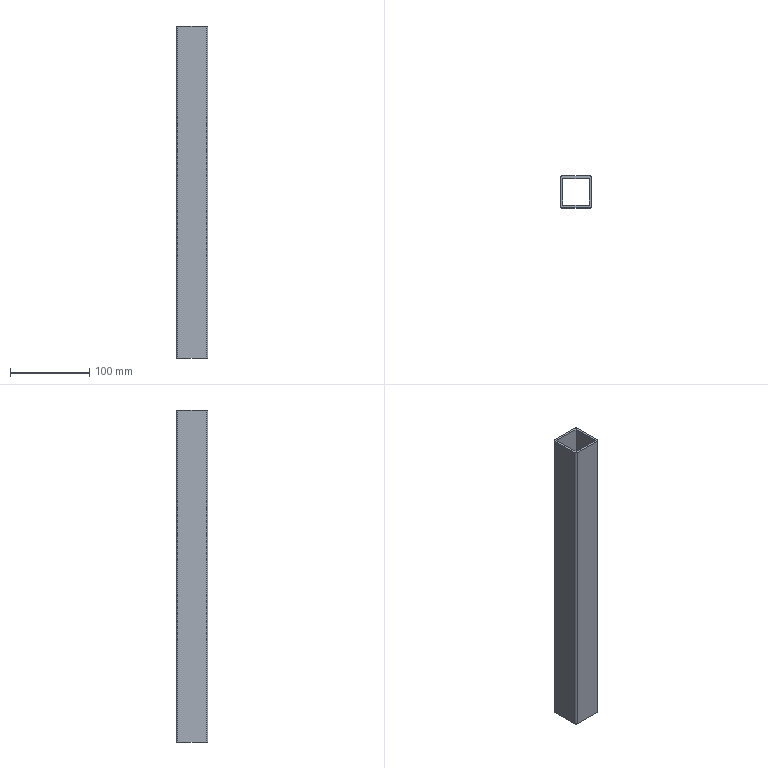Part | STEP file | X77-09108 | 1 solid | 14 faces | box 40 x 40 x 420 mm | volume 185038 mm3 | plane 10 | cylinder 4 | commonest cylinder face diameters 4 x4
STEP:
#1=CARTESIAN_POINT('',(0.,2.,420.));
#2=VERTEX_POINT('',#1);
#3=CARTESIAN_POINT('',(2.,0.,420.));
#4=VERTEX_POINT('',#3);
#5=CARTESIAN_POINT('',(2.,2.,420.));
#6=DIRECTION('',(0.,0.,1.));
#7=DIRECTION('',(1.,0.,0.));
#8=AXIS2_PLACEMENT_3D('',#5,#6,#7);
#9=CIRCLE('',#8,2.);
#10=EDGE_CURVE('',#2,#4,#9,.T.);
#11=ORIENTED_EDGE('',*,*,#10,.T.);
#12=CARTESIAN_POINT('',(38.,0.,420.));
#13=VERTEX_POINT('',#12);
#14=CARTESIAN_POINT('',(2.,0.,420.));
#15=DIRECTION('',(1.,0.,0.));
#16=VECTOR('',#15,1000.);
#17=LINE('',#14,#16);
#18=EDGE_CURVE('',#4,#13,#17,.T.);
#19=ORIENTED_EDGE('',*,*,#18,.T.);
#20=CARTESIAN_POINT('',(40.,2.,420.));
#21=VERTEX_POINT('',#20);
#22=CARTESIAN_POINT('',(38.,2.,420.));
#23=DIRECTION('',(0.,0.,1.));
#24=DIRECTION('',(1.,0.,0.));
#25=AXIS2_PLACEMENT_3D('',#22,#23,#24);
#26=CIRCLE('',#25,2.);
#27=EDGE_CURVE('',#13,#21,#26,.T.);
#28=ORIENTED_EDGE('',*,*,#27,.T.);
#29=CARTESIAN_POINT('',(40.,38.,420.));
#30=VERTEX_POINT('',#29);
#31=CARTESIAN_POINT('',(40.,2.,420.));
#32=DIRECTION('',(0.,1.,0.));
#33=VECTOR('',#32,1000.);
#34=LINE('',#31,#33);
#35=EDGE_CURVE('',#21,#30,#34,.T.);
#36=ORIENTED_EDGE('',*,*,#35,.T.);
#37=CARTESIAN_POINT('',(38.,40.,420.));
#38=VERTEX_POINT('',#37);
#39=CARTESIAN_POINT('',(38.,38.,420.));
#40=DIRECTION('',(0.,0.,1.));
#41=DIRECTION('',(1.,0.,0.));
#42=AXIS2_PLACEMENT_3D('',#39,#40,#41);
#43=CIRCLE('',#42,2.);
#44=EDGE_CURVE('',#30,#38,#43,.T.);
#45=ORIENTED_EDGE('',*,*,#44,.T.);
#46=CARTESIAN_POINT('',(2.,40.,420.));
#47=VERTEX_POINT('',#46);
#48=CARTESIAN_POINT('',(2.,40.,420.));
#49=DIRECTION('',(-1.,0.,0.));
#50=VECTOR('',#49,1000.);
#51=LINE('',#48,#50);
#52=EDGE_CURVE('',#38,#47,#51,.T.);
#53=ORIENTED_EDGE('',*,*,#52,.T.);
#54=CARTESIAN_POINT('',(0.,38.,420.));
#55=VERTEX_POINT('',#54);
#56=CARTESIAN_POINT('',(2.,38.,420.));
#57=DIRECTION('',(0.,0.,1.));
#58=DIRECTION('',(-1.,0.,0.));
#59=AXIS2_PLACEMENT_3D('',#56,#57,#58);
#60=CIRCLE('',#59,2.);
#61=EDGE_CURVE('',#47,#55,#60,.T.);
#62=ORIENTED_EDGE('',*,*,#61,.T.);
#63=CARTESIAN_POINT('',(0.,2.,420.));
#64=DIRECTION('',(0.,-1.,0.));
#65=VECTOR('',#64,1000.);
#66=LINE('',#63,#65);
#67=EDGE_CURVE('',#55,#2,#66,.T.);
#68=ORIENTED_EDGE('',*,*,#67,.T.);
#69=EDGE_LOOP('',(#11,#19,#28,#36,#45,#53,#62,#68));
#70=FACE_OUTER_BOUND('',#69,.T.);
#71=CARTESIAN_POINT('',(3.,3.,420.));
#72=VERTEX_POINT('',#71);
#73=CARTESIAN_POINT('',(37.,3.,420.));
#74=VERTEX_POINT('',#73);
#75=CARTESIAN_POINT('',(3.,3.,420.));
#76=DIRECTION('',(1.,0.,0.));
#77=VECTOR('',#76,1000.);
#78=LINE('',#75,#77);
#79=EDGE_CURVE('',#72,#74,#78,.T.);
#80=ORIENTED_EDGE('',*,*,#79,.F.);
#81=CARTESIAN_POINT('',(3.,37.,420.));
#82=VERTEX_POINT('',#81);
#83=CARTESIAN_POINT('',(3.,3.,420.));
#84=DIRECTION('',(0.,-1.,0.));
#85=VECTOR('',#84,1000.);
#86=LINE('',#83,#85);
#87=EDGE_CURVE('',#82,#72,#86,.T.);
#88=ORIENTED_EDGE('',*,*,#87,.F.);
#89=CARTESIAN_POINT('',(37.,37.,420.));
#90=VERTEX_POINT('',#89);
#91=CARTESIAN_POINT('',(3.,37.,420.));
#92=DIRECTION('',(-1.,0.,0.));
#93=VECTOR('',#92,1000.);
#94=LINE('',#91,#93);
#95=EDGE_CURVE('',#90,#82,#94,.T.);
#96=ORIENTED_EDGE('',*,*,#95,.F.);
#97=CARTESIAN_POINT('',(37.,3.,420.));
#98=DIRECTION('',(0.,1.,0.));
#99=VECTOR('',#98,1000.);
#100=LINE('',#97,#99);
#101=EDGE_CURVE('',#74,#90,#100,.T.);
#102=ORIENTED_EDGE('',*,*,#101,.F.);
#103=EDGE_LOOP('',(#80,#88,#96,#102));
#104=FACE_BOUND('',#103,.T.);
#105=CARTESIAN_POINT('',(2.,2.,420.));
#106=DIRECTION('',(0.,0.,1.));
#107=DIRECTION('',(1.,0.,0.));
#108=AXIS2_PLACEMENT_3D('',#105,#106,#107);
#109=PLANE('',#108);
#110=ADVANCED_FACE('',(#70,#104),#109,.T.);
#111=CARTESIAN_POINT('',(0.,2.,0.));
#112=VERTEX_POINT('',#111);
#113=CARTESIAN_POINT('',(2.,0.,0.));
#114=VERTEX_POINT('',#113);
#115=CARTESIAN_POINT('',(2.,2.,0.));
#116=DIRECTION('',(0.,0.,1.));
#117=DIRECTION('',(1.,0.,0.));
#118=AXIS2_PLACEMENT_3D('',#115,#116,#117);
#119=CIRCLE('',#118,2.);
#120=EDGE_CURVE('',#112,#114,#119,.T.);
#121=ORIENTED_EDGE('',*,*,#120,.F.);
#122=CARTESIAN_POINT('',(0.,38.,0.));
#123=VERTEX_POINT('',#122);
#124=CARTESIAN_POINT('',(0.,2.,0.));
#125=DIRECTION('',(0.,-1.,0.));
#126=VECTOR('',#125,1000.);
#127=LINE('',#124,#126);
#128=EDGE_CURVE('',#123,#112,#127,.T.);
#129=ORIENTED_EDGE('',*,*,#128,.F.);
#130=CARTESIAN_POINT('',(2.,40.,0.));
#131=VERTEX_POINT('',#130);
#132=CARTESIAN_POINT('',(2.,38.,0.));
#133=DIRECTION('',(0.,0.,1.));
#134=DIRECTION('',(-1.,0.,0.));
#135=AXIS2_PLACEMENT_3D('',#132,#133,#134);
#136=CIRCLE('',#135,2.);
#137=EDGE_CURVE('',#131,#123,#136,.T.);
#138=ORIENTED_EDGE('',*,*,#137,.F.);
#139=CARTESIAN_POINT('',(38.,40.,0.));
#140=VERTEX_POINT('',#139);
#141=CARTESIAN_POINT('',(2.,40.,0.));
#142=DIRECTION('',(-1.,0.,0.));
#143=VECTOR('',#142,1000.);
#144=LINE('',#141,#143);
#145=EDGE_CURVE('',#140,#131,#144,.T.);
#146=ORIENTED_EDGE('',*,*,#145,.F.);
#147=CARTESIAN_POINT('',(40.,38.,0.));
#148=VERTEX_POINT('',#147);
#149=CARTESIAN_POINT('',(38.,38.,0.));
#150=DIRECTION('',(0.,0.,1.));
#151=DIRECTION('',(1.,0.,0.));
#152=AXIS2_PLACEMENT_3D('',#149,#150,#151);
#153=CIRCLE('',#152,2.);
#154=EDGE_CURVE('',#148,#140,#153,.T.);
#155=ORIENTED_EDGE('',*,*,#154,.F.);
#156=CARTESIAN_POINT('',(40.,2.,0.));
#157=VERTEX_POINT('',#156);
#158=CARTESIAN_POINT('',(40.,2.,0.));
#159=DIRECTION('',(0.,1.,0.));
#160=VECTOR('',#159,1000.);
#161=LINE('',#158,#160);
#162=EDGE_CURVE('',#157,#148,#161,.T.);
#163=ORIENTED_EDGE('',*,*,#162,.F.);
#164=CARTESIAN_POINT('',(38.,0.,0.));
#165=VERTEX_POINT('',#164);
#166=CARTESIAN_POINT('',(38.,2.,0.));
#167=DIRECTION('',(0.,0.,1.));
#168=DIRECTION('',(1.,0.,0.));
#169=AXIS2_PLACEMENT_3D('',#166,#167,#168);
#170=CIRCLE('',#169,2.);
#171=EDGE_CURVE('',#165,#157,#170,.T.);
#172=ORIENTED_EDGE('',*,*,#171,.F.);
#173=CARTESIAN_POINT('',(2.,0.,0.));
#174=DIRECTION('',(1.,0.,0.));
#175=VECTOR('',#174,1000.);
#176=LINE('',#173,#175);
#177=EDGE_CURVE('',#114,#165,#176,.T.);
#178=ORIENTED_EDGE('',*,*,#177,.F.);
#179=EDGE_LOOP('',(#121,#129,#138,#146,#155,#163,#172,#178));
#180=FACE_OUTER_BOUND('',#179,.T.);
#181=CARTESIAN_POINT('',(3.,37.,0.));
#182=VERTEX_POINT('',#181);
#183=CARTESIAN_POINT('',(3.,3.,0.));
#184=VERTEX_POINT('',#183);
#185=CARTESIAN_POINT('',(3.,3.,0.));
#186=DIRECTION('',(0.,-1.,0.));
#187=VECTOR('',#186,1000.);
#188=LINE('',#185,#187);
#189=EDGE_CURVE('',#182,#184,#188,.T.);
#190=ORIENTED_EDGE('',*,*,#189,.T.);
#191=CARTESIAN_POINT('',(37.,3.,0.));
#192=VERTEX_POINT('',#191);
#193=CARTESIAN_POINT('',(3.,3.,0.));
#194=DIRECTION('',(1.,0.,0.));
#195=VECTOR('',#194,1000.);
#196=LINE('',#193,#195);
#197=EDGE_CURVE('',#184,#192,#196,.T.);
#198=ORIENTED_EDGE('',*,*,#197,.T.);
#199=CARTESIAN_POINT('',(37.,37.,0.));
#200=VERTEX_POINT('',#199);
#201=CARTESIAN_POINT('',(37.,3.,0.));
#202=DIRECTION('',(0.,1.,0.));
#203=VECTOR('',#202,1000.);
#204=LINE('',#201,#203);
#205=EDGE_CURVE('',#192,#200,#204,.T.);
#206=ORIENTED_EDGE('',*,*,#205,.T.);
#207=CARTESIAN_POINT('',(3.,37.,0.));
#208=DIRECTION('',(-1.,0.,0.));
#209=VECTOR('',#208,1000.);
#210=LINE('',#207,#209);
#211=EDGE_CURVE('',#200,#182,#210,.T.);
#212=ORIENTED_EDGE('',*,*,#211,.T.);
#213=EDGE_LOOP('',(#190,#198,#206,#212));
#214=FACE_BOUND('',#213,.T.);
#215=CARTESIAN_POINT('',(2.,2.,0.));
#216=DIRECTION('',(0.,0.,1.));
#217=DIRECTION('',(1.,0.,0.));
#218=AXIS2_PLACEMENT_3D('',#215,#216,#217);
#219=PLANE('',#218);
#220=ADVANCED_FACE('',(#180,#214),#219,.F.);
#221=ORIENTED_EDGE('',*,*,#120,.T.);
#222=CARTESIAN_POINT('',(2.,0.,420.));
#223=DIRECTION('',(0.,0.,-1.));
#224=VECTOR('',#223,1000.);
#225=LINE('',#222,#224);
#226=EDGE_CURVE('',#4,#114,#225,.T.);
#227=ORIENTED_EDGE('',*,*,#226,.F.);
#228=ORIENTED_EDGE('',*,*,#10,.F.);
#229=CARTESIAN_POINT('',(0.,2.,420.));
#230=DIRECTION('',(0.,0.,-1.));
#231=VECTOR('',#230,1000.);
#232=LINE('',#229,#231);
#233=EDGE_CURVE('',#2,#112,#232,.T.);
#234=ORIENTED_EDGE('',*,*,#233,.T.);
#235=EDGE_LOOP('',(#221,#227,#228,#234));
#236=FACE_OUTER_BOUND('',#235,.T.);
#237=CARTESIAN_POINT('',(2.,2.,420.));
#238=DIRECTION('',(0.,0.,-1.));
#239=DIRECTION('',(-1.,0.,0.));
#240=AXIS2_PLACEMENT_3D('',#237,#238,#239);
#241=CYLINDRICAL_SURFACE('',#240,2.);
#242=ADVANCED_FACE('',(#236),#241,.T.);
#243=ORIENTED_EDGE('',*,*,#177,.T.);
#244=CARTESIAN_POINT('',(38.,0.,420.));
#245=DIRECTION('',(0.,0.,-1.));
#246=VECTOR('',#245,1000.);
#247=LINE('',#244,#246);
#248=EDGE_CURVE('',#13,#165,#247,.T.);
#249=ORIENTED_EDGE('',*,*,#248,.F.);
#250=ORIENTED_EDGE('',*,*,#18,.F.);
#251=ORIENTED_EDGE('',*,*,#226,.T.);
#252=EDGE_LOOP('',(#243,#249,#250,#251));
#253=FACE_OUTER_BOUND('',#252,.T.);
#254=CARTESIAN_POINT('',(2.,0.,420.));
#255=DIRECTION('',(0.,1.,0.));
#256=DIRECTION('',(0.,0.,1.));
#257=AXIS2_PLACEMENT_3D('',#254,#255,#256);
#258=PLANE('',#257);
#259=ADVANCED_FACE('',(#253),#258,.F.);
#260=ORIENTED_EDGE('',*,*,#171,.T.);
#261=CARTESIAN_POINT('',(40.,2.,420.));
#262=DIRECTION('',(0.,0.,-1.));
#263=VECTOR('',#262,1000.);
#264=LINE('',#261,#263);
#265=EDGE_CURVE('',#21,#157,#264,.T.);
#266=ORIENTED_EDGE('',*,*,#265,.F.);
#267=ORIENTED_EDGE('',*,*,#27,.F.);
#268=ORIENTED_EDGE('',*,*,#248,.T.);
#269=EDGE_LOOP('',(#260,#266,#267,#268));
#270=FACE_OUTER_BOUND('',#269,.T.);
#271=CARTESIAN_POINT('',(38.,2.,420.));
#272=DIRECTION('',(0.,0.,-1.));
#273=DIRECTION('',(-1.,0.,0.));
#274=AXIS2_PLACEMENT_3D('',#271,#272,#273);
#275=CYLINDRICAL_SURFACE('',#274,2.);
#276=ADVANCED_FACE('',(#270),#275,.T.);
#277=ORIENTED_EDGE('',*,*,#162,.T.);
#278=CARTESIAN_POINT('',(40.,38.,420.));
#279=DIRECTION('',(0.,0.,-1.));
#280=VECTOR('',#279,1000.);
#281=LINE('',#278,#280);
#282=EDGE_CURVE('',#30,#148,#281,.T.);
#283=ORIENTED_EDGE('',*,*,#282,.F.);
#284=ORIENTED_EDGE('',*,*,#35,.F.);
#285=ORIENTED_EDGE('',*,*,#265,.T.);
#286=EDGE_LOOP('',(#277,#283,#284,#285));
#287=FACE_OUTER_BOUND('',#286,.T.);
#288=CARTESIAN_POINT('',(40.,2.,420.));
#289=DIRECTION('',(-1.,0.,0.));
#290=DIRECTION('',(0.,-1.,0.));
#291=AXIS2_PLACEMENT_3D('',#288,#289,#290);
#292=PLANE('',#291);
#293=ADVANCED_FACE('',(#287),#292,.F.);
#294=ORIENTED_EDGE('',*,*,#154,.T.);
#295=CARTESIAN_POINT('',(38.,40.,420.));
#296=DIRECTION('',(0.,0.,-1.));
#297=VECTOR('',#296,1000.);
#298=LINE('',#295,#297);
#299=EDGE_CURVE('',#38,#140,#298,.T.);
#300=ORIENTED_EDGE('',*,*,#299,.F.);
#301=ORIENTED_EDGE('',*,*,#44,.F.);
#302=ORIENTED_EDGE('',*,*,#282,.T.);
#303=EDGE_LOOP('',(#294,#300,#301,#302));
#304=FACE_OUTER_BOUND('',#303,.T.);
#305=CARTESIAN_POINT('',(38.,38.,420.));
#306=DIRECTION('',(0.,0.,-1.));
#307=DIRECTION('',(-1.,0.,0.));
#308=AXIS2_PLACEMENT_3D('',#305,#306,#307);
#309=CYLINDRICAL_SURFACE('',#308,2.);
#310=ADVANCED_FACE('',(#304),#309,.T.);
#311=ORIENTED_EDGE('',*,*,#145,.T.);
#312=CARTESIAN_POINT('',(2.,40.,420.));
#313=DIRECTION('',(0.,0.,-1.));
#314=VECTOR('',#313,1000.);
#315=LINE('',#312,#314);
#316=EDGE_CURVE('',#47,#131,#315,.T.);
#317=ORIENTED_EDGE('',*,*,#316,.F.);
#318=ORIENTED_EDGE('',*,*,#52,.F.);
#319=ORIENTED_EDGE('',*,*,#299,.T.);
#320=EDGE_LOOP('',(#311,#317,#318,#319));
#321=FACE_OUTER_BOUND('',#320,.T.);
#322=CARTESIAN_POINT('',(2.,40.,420.));
#323=DIRECTION('',(0.,-1.,0.));
#324=DIRECTION('',(0.,0.,-1.));
#325=AXIS2_PLACEMENT_3D('',#322,#323,#324);
#326=PLANE('',#325);
#327=ADVANCED_FACE('',(#321),#326,.F.);
#328=ORIENTED_EDGE('',*,*,#137,.T.);
#329=CARTESIAN_POINT('',(0.,38.,420.));
#330=DIRECTION('',(0.,0.,-1.));
#331=VECTOR('',#330,1000.);
#332=LINE('',#329,#331);
#333=EDGE_CURVE('',#55,#123,#332,.T.);
#334=ORIENTED_EDGE('',*,*,#333,.F.);
#335=ORIENTED_EDGE('',*,*,#61,.F.);
#336=ORIENTED_EDGE('',*,*,#316,.T.);
#337=EDGE_LOOP('',(#328,#334,#335,#336));
#338=FACE_OUTER_BOUND('',#337,.T.);
#339=CARTESIAN_POINT('',(2.,38.,420.));
#340=DIRECTION('',(0.,0.,-1.));
#341=DIRECTION('',(-1.,0.,0.));
#342=AXIS2_PLACEMENT_3D('',#339,#340,#341);
#343=CYLINDRICAL_SURFACE('',#342,2.);
#344=ADVANCED_FACE('',(#338),#343,.T.);
#345=ORIENTED_EDGE('',*,*,#128,.T.);
#346=ORIENTED_EDGE('',*,*,#233,.F.);
#347=ORIENTED_EDGE('',*,*,#67,.F.);
#348=ORIENTED_EDGE('',*,*,#333,.T.);
#349=EDGE_LOOP('',(#345,#346,#347,#348));
#350=FACE_OUTER_BOUND('',#349,.T.);
#351=CARTESIAN_POINT('',(0.,2.,420.));
#352=DIRECTION('',(1.,0.,0.));
#353=DIRECTION('',(0.,1.,0.));
#354=AXIS2_PLACEMENT_3D('',#351,#352,#353);
#355=PLANE('',#354);
#356=ADVANCED_FACE('',(#350),#355,.F.);
#357=ORIENTED_EDGE('',*,*,#189,.F.);
#358=CARTESIAN_POINT('',(3.,37.,420.));
#359=DIRECTION('',(0.,0.,-1.));
#360=VECTOR('',#359,1000.);
#361=LINE('',#358,#360);
#362=EDGE_CURVE('',#82,#182,#361,.T.);
#363=ORIENTED_EDGE('',*,*,#362,.F.);
#364=ORIENTED_EDGE('',*,*,#87,.T.);
#365=CARTESIAN_POINT('',(3.,3.,420.));
#366=DIRECTION('',(0.,0.,-1.));
#367=VECTOR('',#366,1000.);
#368=LINE('',#365,#367);
#369=EDGE_CURVE('',#72,#184,#368,.T.);
#370=ORIENTED_EDGE('',*,*,#369,.T.);
#371=EDGE_LOOP('',(#357,#363,#364,#370));
#372=FACE_OUTER_BOUND('',#371,.T.);
#373=CARTESIAN_POINT('',(3.,3.,420.));
#374=DIRECTION('',(1.,0.,0.));
#375=DIRECTION('',(0.,0.,-1.));
#376=AXIS2_PLACEMENT_3D('',#373,#374,#375);
#377=PLANE('',#376);
#378=ADVANCED_FACE('',(#372),#377,.T.);
#379=ORIENTED_EDGE('',*,*,#197,.F.);
#380=ORIENTED_EDGE('',*,*,#369,.F.);
#381=ORIENTED_EDGE('',*,*,#79,.T.);
#382=CARTESIAN_POINT('',(37.,3.,420.));
#383=DIRECTION('',(0.,0.,-1.));
#384=VECTOR('',#383,1000.);
#385=LINE('',#382,#384);
#386=EDGE_CURVE('',#74,#192,#385,.T.);
#387=ORIENTED_EDGE('',*,*,#386,.T.);
#388=EDGE_LOOP('',(#379,#380,#381,#387));
#389=FACE_OUTER_BOUND('',#388,.T.);
#390=CARTESIAN_POINT('',(3.,3.,420.));
#391=DIRECTION('',(0.,1.,0.));
#392=DIRECTION('',(0.,0.,1.));
#393=AXIS2_PLACEMENT_3D('',#390,#391,#392);
#394=PLANE('',#393);
#395=ADVANCED_FACE('',(#389),#394,.T.);
#396=ORIENTED_EDGE('',*,*,#205,.F.);
#397=ORIENTED_EDGE('',*,*,#386,.F.);
#398=ORIENTED_EDGE('',*,*,#101,.T.);
#399=CARTESIAN_POINT('',(37.,37.,420.));
#400=DIRECTION('',(0.,0.,-1.));
#401=VECTOR('',#400,1000.);
#402=LINE('',#399,#401);
#403=EDGE_CURVE('',#90,#200,#402,.T.);
#404=ORIENTED_EDGE('',*,*,#403,.T.);
#405=EDGE_LOOP('',(#396,#397,#398,#404));
#406=FACE_OUTER_BOUND('',#405,.T.);
#407=CARTESIAN_POINT('',(37.,3.,420.));
#408=DIRECTION('',(-1.,0.,0.));
#409=DIRECTION('',(0.,0.,1.));
#410=AXIS2_PLACEMENT_3D('',#407,#408,#409);
#411=PLANE('',#410);
#412=ADVANCED_FACE('',(#406),#411,.T.);
#413=ORIENTED_EDGE('',*,*,#211,.F.);
#414=ORIENTED_EDGE('',*,*,#403,.F.);
#415=ORIENTED_EDGE('',*,*,#95,.T.);
#416=ORIENTED_EDGE('',*,*,#362,.T.);
#417=EDGE_LOOP('',(#413,#414,#415,#416));
#418=FACE_OUTER_BOUND('',#417,.T.);
#419=CARTESIAN_POINT('',(3.,37.,420.));
#420=DIRECTION('',(0.,-1.,0.));
#421=DIRECTION('',(0.,0.,-1.));
#422=AXIS2_PLACEMENT_3D('',#419,#420,#421);
#423=PLANE('',#422);
#424=ADVANCED_FACE('',(#418),#423,.T.);
#425=CLOSED_SHELL('',(#110,#220,#242,#259,#276,#293,#310,#327,#344,#356,#378,#395,#412,#424));
#426=MANIFOLD_SOLID_BREP('',#425);
#427=CARTESIAN_POINT('',(0.,0.,0.));
#428=DIRECTION('',(0.,0.,1.));
#429=DIRECTION('',(1.,0.,0.));
#430=AXIS2_PLACEMENT_3D('',#427,#428,#429);
#431=(LENGTH_UNIT()NAMED_UNIT(*)SI_UNIT(.MILLI.,.METRE.));
#432=UNCERTAINTY_MEASURE_WITH_UNIT(LENGTH_MEASURE(0.00001),#431,'','');
#433=(NAMED_UNIT(*)PLANE_ANGLE_UNIT()SI_UNIT($,.RADIAN.));
#434=(NAMED_UNIT(*)SI_UNIT($,.STERADIAN.)SOLID_ANGLE_UNIT());
#435=(GEOMETRIC_REPRESENTATION_CONTEXT(3)GLOBAL_UNCERTAINTY_ASSIGNED_CONTEXT((#432))GLOBAL_UNIT_ASSIGNED_CONTEXT((#431,#433,#434))REPRESENTATION_CONTEXT('',''));
#436=ADVANCED_BREP_SHAPE_REPRESENTATION('',(#426,#430),#435);